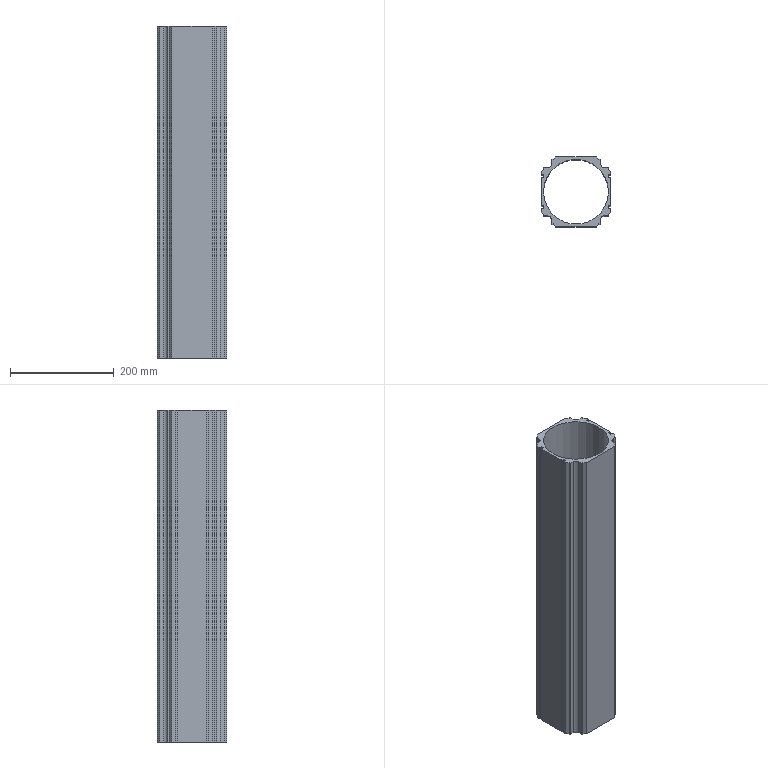Part | SolidWorks | features Extrusion 1 | 1 solid | 84 faces | box 134 x 134 x 640 mm | volume 2400423 mm3 | plane 70 | spline 12 | cylinder 2 | commonest cylinder face diameters 125 x2